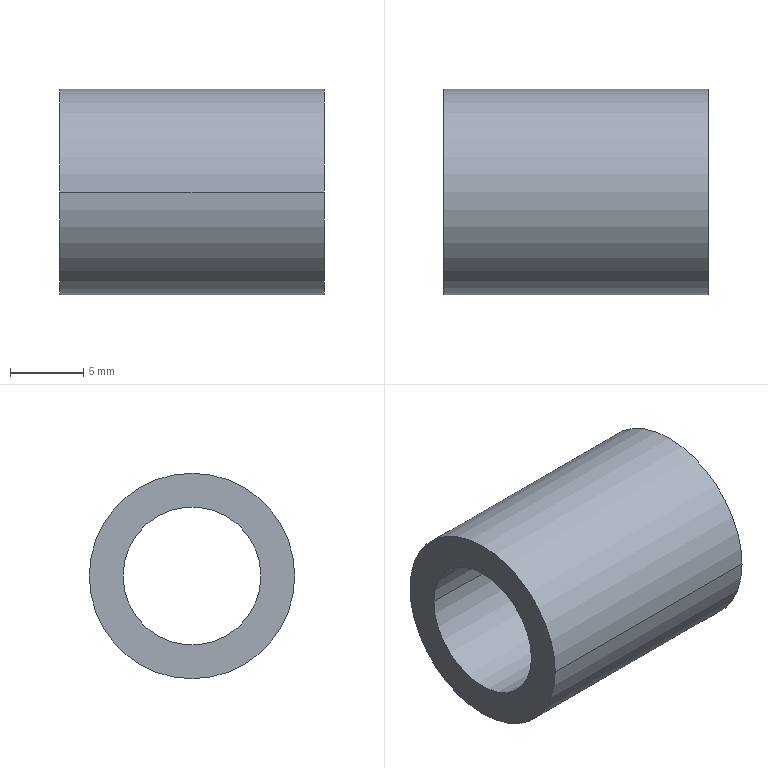Part | STEP file | BREP_5 | 1 solid | 6 faces | box 18 x 14 x 14 mm | volume 1522 mm3 | cylinder 4 | plane 2 | commonest cylinder face diameters 9.4 x2 14 x2
STEP:
#1=CARTESIAN_POINT('',(0.,0.,0.));
#2=DIRECTION('',(0.,0.,1.));
#3=DIRECTION('',(1.,0.,0.));
#4=AXIS2_PLACEMENT_3D('',#1,#2,#3);
#5=CARTESIAN_POINT('',(-69.04,-7.,0.));
#6=VERTEX_POINT('',#5);
#7=CARTESIAN_POINT('',(-69.04,7.,0.));
#8=VERTEX_POINT('',#7);
#9=CARTESIAN_POINT('',(-69.04,0.,0.));
#10=DIRECTION('',(1.,0.,0.));
#11=DIRECTION('',(0.,-1.,0.));
#12=AXIS2_PLACEMENT_3D('',#9,#10,#11);
#13=CIRCLE('',#12,7.);
#14=CARTESIAN_POINT('',(-69.04,-7.,7.));
#15=DIRECTION('',(1.,0.,0.));
#16=DIRECTION('',(0.,1.,0.));
#17=AXIS2_PLACEMENT_3D('',#14,#15,#16);
#18=PLANE('',#17);
#19=CARTESIAN_POINT('',(7.,-7.));
#20=DIRECTION('',(-1.,0.));
#21=AXIS2_PLACEMENT_2D('',#19,#20);
#22=CIRCLE('',#21,7.);
#23=(GEOMETRIC_REPRESENTATION_CONTEXT(2)PARAMETRIC_REPRESENTATION_CONTEXT()REPRESENTATION_CONTEXT('',''));
#24=DEFINITIONAL_REPRESENTATION('',(#22),#23);
#25=PCURVE('',#18,#24);
#26=CARTESIAN_POINT('',(-78.04,0.,0.));
#27=DIRECTION('',(-1.,0.,0.));
#28=DIRECTION('',(0.,-1.,0.));
#29=AXIS2_PLACEMENT_3D('',#26,#27,#28);
#30=CYLINDRICAL_SURFACE('',#29,7.);
#31=CARTESIAN_POINT('',(6.283,-9.));
#32=DIRECTION('',(-1.,0.));
#33=VECTOR('',#32,1.);
#34=LINE('',#31,#33);
#35=(GEOMETRIC_REPRESENTATION_CONTEXT(2)PARAMETRIC_REPRESENTATION_CONTEXT()REPRESENTATION_CONTEXT('',''));
#36=DEFINITIONAL_REPRESENTATION('',(#34),#35);
#37=PCURVE('',#30,#36);
#38=SURFACE_CURVE('',#13,(#25,#37),.PCURVE_S1.);
#39=EDGE_CURVE('',#6,#8,#38,.T.);
#40=ORIENTED_EDGE('',*,*,#39,.F.);
#41=CARTESIAN_POINT('',(-69.04,0.,0.));
#42=DIRECTION('',(1.,0.,0.));
#43=DIRECTION('',(0.,1.,0.));
#44=AXIS2_PLACEMENT_3D('',#41,#42,#43);
#45=CIRCLE('',#44,7.);
#46=CARTESIAN_POINT('',(7.,-7.));
#47=DIRECTION('',(1.,0.));
#48=AXIS2_PLACEMENT_2D('',#46,#47);
#49=CIRCLE('',#48,7.);
#50=(GEOMETRIC_REPRESENTATION_CONTEXT(2)PARAMETRIC_REPRESENTATION_CONTEXT()REPRESENTATION_CONTEXT('',''));
#51=DEFINITIONAL_REPRESENTATION('',(#49),#50);
#52=PCURVE('',#18,#51);
#53=CARTESIAN_POINT('',(-78.04,0.,0.));
#54=DIRECTION('',(-1.,0.,0.));
#55=DIRECTION('',(0.,1.,0.));
#56=AXIS2_PLACEMENT_3D('',#53,#54,#55);
#57=CYLINDRICAL_SURFACE('',#56,7.);
#58=CARTESIAN_POINT('',(6.283,-9.));
#59=DIRECTION('',(-1.,0.));
#60=VECTOR('',#59,1.);
#61=LINE('',#58,#60);
#62=(GEOMETRIC_REPRESENTATION_CONTEXT(2)PARAMETRIC_REPRESENTATION_CONTEXT()REPRESENTATION_CONTEXT('',''));
#63=DEFINITIONAL_REPRESENTATION('',(#61),#62);
#64=PCURVE('',#57,#63);
#65=SURFACE_CURVE('',#45,(#52,#64),.PCURVE_S1.);
#66=EDGE_CURVE('',#8,#6,#65,.T.);
#67=ORIENTED_EDGE('',*,*,#66,.F.);
#68=EDGE_LOOP('',(#40,#67));
#69=FACE_BOUND('',#68,.F.);
#70=CARTESIAN_POINT('',(-69.04,4.7,0.));
#71=VERTEX_POINT('',#70);
#72=CARTESIAN_POINT('',(-69.04,-4.7,0.));
#73=VERTEX_POINT('',#72);
#74=CARTESIAN_POINT('',(-69.04,0.,0.));
#75=DIRECTION('',(-1.,0.,0.));
#76=DIRECTION('',(0.,1.,0.));
#77=AXIS2_PLACEMENT_3D('',#74,#75,#76);
#78=CIRCLE('',#77,4.7);
#79=CARTESIAN_POINT('',(11.7,-7.));
#80=CARTESIAN_POINT('',(11.7,-15.141));
#81=CARTESIAN_POINT('',(4.65,-11.07));
#82=CARTESIAN_POINT('',(-2.4,-7.));
#83=CARTESIAN_POINT('',(4.65,-2.93));
#84=CARTESIAN_POINT('',(11.7,1.141));
#85=CARTESIAN_POINT('',(11.7,-7.));
#86=(BOUNDED_CURVE()B_SPLINE_CURVE(2,(#79,#80,#81,#82,#83,#84,#85),.UNSPECIFIED.,.T.,.F.)B_SPLINE_CURVE_WITH_KNOTS((1,2,2,2,2,1),(-2.094,0.,2.094,4.189,6.283,8.378),.UNSPECIFIED.)CURVE()GEOMETRIC_REPRESENTATION_ITEM()RATIONAL_B_SPLINE_CURVE((1.,0.5,1.,0.5,1.,0.5,1.))REPRESENTATION_ITEM(''));
#87=(GEOMETRIC_REPRESENTATION_CONTEXT(2)PARAMETRIC_REPRESENTATION_CONTEXT()REPRESENTATION_CONTEXT('',''));
#88=DEFINITIONAL_REPRESENTATION('',(#86),#87);
#89=PCURVE('',#18,#88);
#90=CARTESIAN_POINT('',(-78.04,0.,0.));
#91=DIRECTION('',(-1.,0.,0.));
#92=DIRECTION('',(0.,1.,0.));
#93=AXIS2_PLACEMENT_3D('',#90,#91,#92);
#94=CYLINDRICAL_SURFACE('',#93,4.7);
#95=CARTESIAN_POINT('',(0.,-9.));
#96=DIRECTION('',(1.,0.));
#97=VECTOR('',#96,1.);
#98=LINE('',#95,#97);
#99=(GEOMETRIC_REPRESENTATION_CONTEXT(2)PARAMETRIC_REPRESENTATION_CONTEXT()REPRESENTATION_CONTEXT('',''));
#100=DEFINITIONAL_REPRESENTATION('',(#98),#99);
#101=PCURVE('',#94,#100);
#102=SURFACE_CURVE('',#78,(#89,#101),.PCURVE_S1.);
#103=EDGE_CURVE('',#71,#73,#102,.T.);
#104=ORIENTED_EDGE('',*,*,#103,.F.);
#105=CARTESIAN_POINT('',(-69.04,0.,0.));
#106=DIRECTION('',(-1.,0.,0.));
#107=DIRECTION('',(0.,-1.,0.));
#108=AXIS2_PLACEMENT_3D('',#105,#106,#107);
#109=CIRCLE('',#108,4.7);
#110=CARTESIAN_POINT('',(2.3,-7.));
#111=CARTESIAN_POINT('',(2.3,1.141));
#112=CARTESIAN_POINT('',(9.35,-2.93));
#113=CARTESIAN_POINT('',(16.4,-7.));
#114=CARTESIAN_POINT('',(9.35,-11.07));
#115=CARTESIAN_POINT('',(2.3,-15.141));
#116=CARTESIAN_POINT('',(2.3,-7.));
#117=(BOUNDED_CURVE()B_SPLINE_CURVE(2,(#110,#111,#112,#113,#114,#115,#116),.UNSPECIFIED.,.T.,.F.)B_SPLINE_CURVE_WITH_KNOTS((1,2,2,2,2,1),(-2.094,0.,2.094,4.189,6.283,8.378),.UNSPECIFIED.)CURVE()GEOMETRIC_REPRESENTATION_ITEM()RATIONAL_B_SPLINE_CURVE((1.,0.5,1.,0.5,1.,0.5,1.))REPRESENTATION_ITEM(''));
#118=(GEOMETRIC_REPRESENTATION_CONTEXT(2)PARAMETRIC_REPRESENTATION_CONTEXT()REPRESENTATION_CONTEXT('',''));
#119=DEFINITIONAL_REPRESENTATION('',(#117),#118);
#120=PCURVE('',#18,#119);
#121=CARTESIAN_POINT('',(-78.04,0.,0.));
#122=DIRECTION('',(-1.,0.,0.));
#123=DIRECTION('',(0.,-1.,0.));
#124=AXIS2_PLACEMENT_3D('',#121,#122,#123);
#125=CYLINDRICAL_SURFACE('',#124,4.7);
#126=CARTESIAN_POINT('',(0.,-9.));
#127=DIRECTION('',(1.,0.));
#128=VECTOR('',#127,1.);
#129=LINE('',#126,#128);
#130=(GEOMETRIC_REPRESENTATION_CONTEXT(2)PARAMETRIC_REPRESENTATION_CONTEXT()REPRESENTATION_CONTEXT('',''));
#131=DEFINITIONAL_REPRESENTATION('',(#129),#130);
#132=PCURVE('',#125,#131);
#133=SURFACE_CURVE('',#109,(#120,#132),.PCURVE_S1.);
#134=EDGE_CURVE('',#73,#71,#133,.T.);
#135=ORIENTED_EDGE('',*,*,#134,.F.);
#136=EDGE_LOOP('',(#104,#135));
#137=FACE_BOUND('',#136,.F.);
#138=ADVANCED_FACE('',(#69,#137),#18,.T.);
#139=CARTESIAN_POINT('',(-87.04,-7.,0.));
#140=VERTEX_POINT('',#139);
#141=CARTESIAN_POINT('',(-87.04,-7.,0.));
#142=DIRECTION('',(1.,0.,0.));
#143=VECTOR('',#142,1.);
#144=LINE('',#141,#143);
#145=CARTESIAN_POINT('',(6.283,9.));
#146=DIRECTION('',(0.,-1.));
#147=VECTOR('',#146,1.);
#148=LINE('',#145,#147);
#149=(GEOMETRIC_REPRESENTATION_CONTEXT(2)PARAMETRIC_REPRESENTATION_CONTEXT()REPRESENTATION_CONTEXT('',''));
#150=DEFINITIONAL_REPRESENTATION('',(#148),#149);
#151=PCURVE('',#30,#150);
#152=CARTESIAN_POINT('',(3.142,9.));
#153=DIRECTION('',(0.,-1.));
#154=VECTOR('',#153,1.);
#155=LINE('',#152,#154);
#156=(GEOMETRIC_REPRESENTATION_CONTEXT(2)PARAMETRIC_REPRESENTATION_CONTEXT()REPRESENTATION_CONTEXT('',''));
#157=DEFINITIONAL_REPRESENTATION('',(#155),#156);
#158=PCURVE('',#57,#157);
#159=SURFACE_CURVE('',#144,(#151,#158),.PCURVE_S1.);
#160=EDGE_CURVE('',#140,#6,#159,.T.);
#161=ORIENTED_EDGE('',*,*,#160,.F.);
#162=CARTESIAN_POINT('',(-87.04,7.,0.));
#163=VERTEX_POINT('',#162);
#164=CARTESIAN_POINT('',(-87.04,0.,0.));
#165=DIRECTION('',(-1.,0.,0.));
#166=DIRECTION('',(0.,1.,0.));
#167=AXIS2_PLACEMENT_3D('',#164,#165,#166);
#168=CIRCLE('',#167,7.);
#169=CARTESIAN_POINT('',(3.142,9.));
#170=DIRECTION('',(1.,0.));
#171=VECTOR('',#170,1.);
#172=LINE('',#169,#171);
#173=(GEOMETRIC_REPRESENTATION_CONTEXT(2)PARAMETRIC_REPRESENTATION_CONTEXT()REPRESENTATION_CONTEXT('',''));
#174=DEFINITIONAL_REPRESENTATION('',(#172),#173);
#175=PCURVE('',#30,#174);
#176=CARTESIAN_POINT('',(-87.04,-7.,7.));
#177=DIRECTION('',(-1.,0.,0.));
#178=DIRECTION('',(0.,1.,0.));
#179=AXIS2_PLACEMENT_3D('',#176,#177,#178);
#180=PLANE('',#179);
#181=CARTESIAN_POINT('',(7.,7.));
#182=DIRECTION('',(1.,0.));
#183=AXIS2_PLACEMENT_2D('',#181,#182);
#184=CIRCLE('',#183,7.);
#185=(GEOMETRIC_REPRESENTATION_CONTEXT(2)PARAMETRIC_REPRESENTATION_CONTEXT()REPRESENTATION_CONTEXT('',''));
#186=DEFINITIONAL_REPRESENTATION('',(#184),#185);
#187=PCURVE('',#180,#186);
#188=SURFACE_CURVE('',#168,(#175,#187),.PCURVE_S1.);
#189=EDGE_CURVE('',#163,#140,#188,.T.);
#190=ORIENTED_EDGE('',*,*,#189,.F.);
#191=CARTESIAN_POINT('',(-87.04,7.,0.));
#192=DIRECTION('',(1.,0.,0.));
#193=VECTOR('',#192,1.);
#194=LINE('',#191,#193);
#195=CARTESIAN_POINT('',(3.142,9.));
#196=DIRECTION('',(0.,-1.));
#197=VECTOR('',#196,1.);
#198=LINE('',#195,#197);
#199=(GEOMETRIC_REPRESENTATION_CONTEXT(2)PARAMETRIC_REPRESENTATION_CONTEXT()REPRESENTATION_CONTEXT('',''));
#200=DEFINITIONAL_REPRESENTATION('',(#198),#199);
#201=PCURVE('',#30,#200);
#202=CARTESIAN_POINT('',(6.283,9.));
#203=DIRECTION('',(0.,-1.));
#204=VECTOR('',#203,1.);
#205=LINE('',#202,#204);
#206=(GEOMETRIC_REPRESENTATION_CONTEXT(2)PARAMETRIC_REPRESENTATION_CONTEXT()REPRESENTATION_CONTEXT('',''));
#207=DEFINITIONAL_REPRESENTATION('',(#205),#206);
#208=PCURVE('',#57,#207);
#209=SURFACE_CURVE('',#194,(#201,#208),.PCURVE_S1.);
#210=EDGE_CURVE('',#163,#8,#209,.T.);
#211=ORIENTED_EDGE('',*,*,#210,.T.);
#212=ORIENTED_EDGE('',*,*,#39,.F.);
#213=EDGE_LOOP('',(#161,#190,#211,#212));
#214=FACE_BOUND('',#213,.T.);
#215=ADVANCED_FACE('',(#214),#30,.T.);
#216=CARTESIAN_POINT('',(-87.04,0.,0.));
#217=DIRECTION('',(-1.,0.,0.));
#218=DIRECTION('',(0.,-1.,0.));
#219=AXIS2_PLACEMENT_3D('',#216,#217,#218);
#220=CIRCLE('',#219,7.);
#221=CARTESIAN_POINT('',(3.142,9.));
#222=DIRECTION('',(1.,0.));
#223=VECTOR('',#222,1.);
#224=LINE('',#221,#223);
#225=(GEOMETRIC_REPRESENTATION_CONTEXT(2)PARAMETRIC_REPRESENTATION_CONTEXT()REPRESENTATION_CONTEXT('',''));
#226=DEFINITIONAL_REPRESENTATION('',(#224),#225);
#227=PCURVE('',#57,#226);
#228=CARTESIAN_POINT('',(7.,7.));
#229=DIRECTION('',(-1.,0.));
#230=AXIS2_PLACEMENT_2D('',#228,#229);
#231=CIRCLE('',#230,7.);
#232=(GEOMETRIC_REPRESENTATION_CONTEXT(2)PARAMETRIC_REPRESENTATION_CONTEXT()REPRESENTATION_CONTEXT('',''));
#233=DEFINITIONAL_REPRESENTATION('',(#231),#232);
#234=PCURVE('',#180,#233);
#235=SURFACE_CURVE('',#220,(#227,#234),.PCURVE_S1.);
#236=EDGE_CURVE('',#140,#163,#235,.T.);
#237=ORIENTED_EDGE('',*,*,#236,.F.);
#238=ORIENTED_EDGE('',*,*,#160,.T.);
#239=ORIENTED_EDGE('',*,*,#66,.F.);
#240=ORIENTED_EDGE('',*,*,#210,.F.);
#241=EDGE_LOOP('',(#237,#238,#239,#240));
#242=FACE_BOUND('',#241,.T.);
#243=ADVANCED_FACE('',(#242),#57,.T.);
#244=ORIENTED_EDGE('',*,*,#236,.F.);
#245=ORIENTED_EDGE('',*,*,#189,.F.);
#246=EDGE_LOOP('',(#244,#245));
#247=FACE_BOUND('',#246,.F.);
#248=CARTESIAN_POINT('',(-87.04,4.7,0.));
#249=VERTEX_POINT('',#248);
#250=CARTESIAN_POINT('',(-87.04,-4.7,0.));
#251=VERTEX_POINT('',#250);
#252=CARTESIAN_POINT('',(-87.04,0.,0.));
#253=DIRECTION('',(1.,0.,0.));
#254=DIRECTION('',(0.,1.,0.));
#255=AXIS2_PLACEMENT_3D('',#252,#253,#254);
#256=CIRCLE('',#255,4.7);
#257=CARTESIAN_POINT('',(11.7,7.));
#258=CARTESIAN_POINT('',(11.7,-1.141));
#259=CARTESIAN_POINT('',(4.65,2.93));
#260=CARTESIAN_POINT('',(-2.4,7.));
#261=CARTESIAN_POINT('',(4.65,11.07));
#262=CARTESIAN_POINT('',(11.7,15.141));
#263=CARTESIAN_POINT('',(11.7,7.));
#264=(BOUNDED_CURVE()B_SPLINE_CURVE(2,(#257,#258,#259,#260,#261,#262,#263),.UNSPECIFIED.,.T.,.F.)B_SPLINE_CURVE_WITH_KNOTS((1,2,2,2,2,1),(-2.094,0.,2.094,4.189,6.283,8.378),.UNSPECIFIED.)CURVE()GEOMETRIC_REPRESENTATION_ITEM()RATIONAL_B_SPLINE_CURVE((1.,0.5,1.,0.5,1.,0.5,1.))REPRESENTATION_ITEM(''));
#265=(GEOMETRIC_REPRESENTATION_CONTEXT(2)PARAMETRIC_REPRESENTATION_CONTEXT()REPRESENTATION_CONTEXT('',''));
#266=DEFINITIONAL_REPRESENTATION('',(#264),#265);
#267=PCURVE('',#180,#266);
#268=CARTESIAN_POINT('',(3.142,9.));
#269=DIRECTION('',(-1.,0.));
#270=VECTOR('',#269,1.);
#271=LINE('',#268,#270);
#272=(GEOMETRIC_REPRESENTATION_CONTEXT(2)PARAMETRIC_REPRESENTATION_CONTEXT()REPRESENTATION_CONTEXT('',''));
#273=DEFINITIONAL_REPRESENTATION('',(#271),#272);
#274=PCURVE('',#125,#273);
#275=SURFACE_CURVE('',#256,(#267,#274),.PCURVE_S1.);
#276=EDGE_CURVE('',#249,#251,#275,.T.);
#277=ORIENTED_EDGE('',*,*,#276,.F.);
#278=CARTESIAN_POINT('',(-87.04,0.,0.));
#279=DIRECTION('',(1.,0.,0.));
#280=DIRECTION('',(0.,-1.,0.));
#281=AXIS2_PLACEMENT_3D('',#278,#279,#280);
#282=CIRCLE('',#281,4.7);
#283=CARTESIAN_POINT('',(2.3,7.));
#284=CARTESIAN_POINT('',(2.3,15.141));
#285=CARTESIAN_POINT('',(9.35,11.07));
#286=CARTESIAN_POINT('',(16.4,7.));
#287=CARTESIAN_POINT('',(9.35,2.93));
#288=CARTESIAN_POINT('',(2.3,-1.141));
#289=CARTESIAN_POINT('',(2.3,7.));
#290=(BOUNDED_CURVE()B_SPLINE_CURVE(2,(#283,#284,#285,#286,#287,#288,#289),.UNSPECIFIED.,.T.,.F.)B_SPLINE_CURVE_WITH_KNOTS((1,2,2,2,2,1),(-2.094,0.,2.094,4.189,6.283,8.378),.UNSPECIFIED.)CURVE()GEOMETRIC_REPRESENTATION_ITEM()RATIONAL_B_SPLINE_CURVE((1.,0.5,1.,0.5,1.,0.5,1.))REPRESENTATION_ITEM(''));
#291=(GEOMETRIC_REPRESENTATION_CONTEXT(2)PARAMETRIC_REPRESENTATION_CONTEXT()REPRESENTATION_CONTEXT('',''));
#292=DEFINITIONAL_REPRESENTATION('',(#290),#291);
#293=PCURVE('',#180,#292);
#294=CARTESIAN_POINT('',(3.142,9.));
#295=DIRECTION('',(-1.,0.));
#296=VECTOR('',#295,1.);
#297=LINE('',#294,#296);
#298=(GEOMETRIC_REPRESENTATION_CONTEXT(2)PARAMETRIC_REPRESENTATION_CONTEXT()REPRESENTATION_CONTEXT('',''));
#299=DEFINITIONAL_REPRESENTATION('',(#297),#298);
#300=PCURVE('',#94,#299);
#301=SURFACE_CURVE('',#282,(#293,#300),.PCURVE_S1.);
#302=EDGE_CURVE('',#251,#249,#301,.T.);
#303=ORIENTED_EDGE('',*,*,#302,.F.);
#304=EDGE_LOOP('',(#277,#303));
#305=FACE_BOUND('',#304,.F.);
#306=ADVANCED_FACE('',(#247,#305),#180,.T.);
#307=CARTESIAN_POINT('',(-87.04,-4.7,0.));
#308=DIRECTION('',(1.,0.,0.));
#309=VECTOR('',#308,1.);
#310=LINE('',#307,#309);
#311=CARTESIAN_POINT('',(0.,9.));
#312=DIRECTION('',(0.,-1.));
#313=VECTOR('',#312,1.);
#314=LINE('',#311,#313);
#315=(GEOMETRIC_REPRESENTATION_CONTEXT(2)PARAMETRIC_REPRESENTATION_CONTEXT()REPRESENTATION_CONTEXT('',''));
#316=DEFINITIONAL_REPRESENTATION('',(#314),#315);
#317=PCURVE('',#125,#316);
#318=CARTESIAN_POINT('',(3.142,9.));
#319=DIRECTION('',(0.,-1.));
#320=VECTOR('',#319,1.);
#321=LINE('',#318,#320);
#322=(GEOMETRIC_REPRESENTATION_CONTEXT(2)PARAMETRIC_REPRESENTATION_CONTEXT()REPRESENTATION_CONTEXT('',''));
#323=DEFINITIONAL_REPRESENTATION('',(#321),#322);
#324=PCURVE('',#94,#323);
#325=SURFACE_CURVE('',#310,(#317,#324),.PCURVE_S1.);
#326=EDGE_CURVE('',#251,#73,#325,.T.);
#327=ORIENTED_EDGE('',*,*,#326,.T.);
#328=ORIENTED_EDGE('',*,*,#134,.T.);
#329=CARTESIAN_POINT('',(-87.04,4.7,0.));
#330=DIRECTION('',(1.,0.,0.));
#331=VECTOR('',#330,1.);
#332=LINE('',#329,#331);
#333=CARTESIAN_POINT('',(3.142,9.));
#334=DIRECTION('',(0.,-1.));
#335=VECTOR('',#334,1.);
#336=LINE('',#333,#335);
#337=(GEOMETRIC_REPRESENTATION_CONTEXT(2)PARAMETRIC_REPRESENTATION_CONTEXT()REPRESENTATION_CONTEXT('',''));
#338=DEFINITIONAL_REPRESENTATION('',(#336),#337);
#339=PCURVE('',#125,#338);
#340=CARTESIAN_POINT('',(0.,9.));
#341=DIRECTION('',(0.,-1.));
#342=VECTOR('',#341,1.);
#343=LINE('',#340,#342);
#344=(GEOMETRIC_REPRESENTATION_CONTEXT(2)PARAMETRIC_REPRESENTATION_CONTEXT()REPRESENTATION_CONTEXT('',''));
#345=DEFINITIONAL_REPRESENTATION('',(#343),#344);
#346=PCURVE('',#94,#345);
#347=SURFACE_CURVE('',#332,(#339,#346),.PCURVE_S1.);
#348=EDGE_CURVE('',#249,#71,#347,.T.);
#349=ORIENTED_EDGE('',*,*,#348,.F.);
#350=ORIENTED_EDGE('',*,*,#276,.T.);
#351=EDGE_LOOP('',(#327,#328,#349,#350));
#352=FACE_BOUND('',#351,.F.);
#353=ADVANCED_FACE('',(#352),#125,.F.);
#354=ORIENTED_EDGE('',*,*,#103,.T.);
#355=ORIENTED_EDGE('',*,*,#326,.F.);
#356=ORIENTED_EDGE('',*,*,#302,.T.);
#357=ORIENTED_EDGE('',*,*,#348,.T.);
#358=EDGE_LOOP('',(#354,#355,#356,#357));
#359=FACE_BOUND('',#358,.F.);
#360=ADVANCED_FACE('',(#359),#94,.F.);
#361=CLOSED_SHELL('',(#138,#215,#243,#306,#353,#360));
#362=MANIFOLD_SOLID_BREP('',#361);
#363=(LENGTH_UNIT()NAMED_UNIT(*)SI_UNIT(.MILLI.,.METRE.));
#364=UNCERTAINTY_MEASURE_WITH_UNIT(LENGTH_MEASURE(0.0000001),#363,'','');
#365=(NAMED_UNIT(*)PLANE_ANGLE_UNIT()SI_UNIT($,.RADIAN.));
#366=(NAMED_UNIT(*)SI_UNIT($,.STERADIAN.)SOLID_ANGLE_UNIT());
#367=(GEOMETRIC_REPRESENTATION_CONTEXT(3)GLOBAL_UNCERTAINTY_ASSIGNED_CONTEXT((#364))GLOBAL_UNIT_ASSIGNED_CONTEXT((#363,#365,#366))REPRESENTATION_CONTEXT('',''));
#368=ADVANCED_BREP_SHAPE_REPRESENTATION('',(#4,#362),#367);